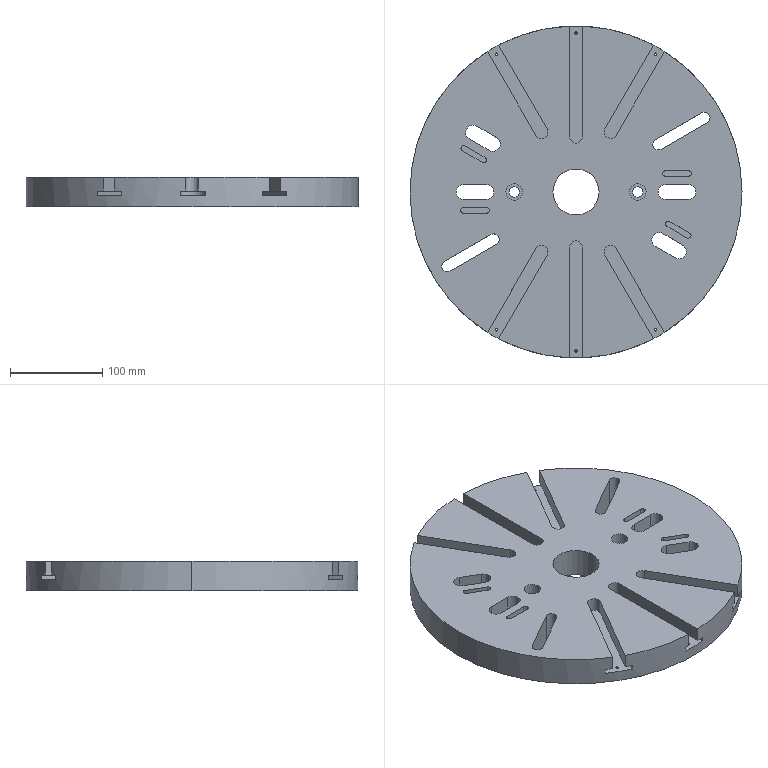Part | SolidWorks | features ICE 9, Extrusion 1 | 1 solid | 164 faces | box 360 x 360 x 32 mm | volume 2735603 mm3 | cylinder 86 | plane 78 | commonest cylinder face diameters 30 x20 2.75 x12 6 x12 16 x12 11 x8 14 x8